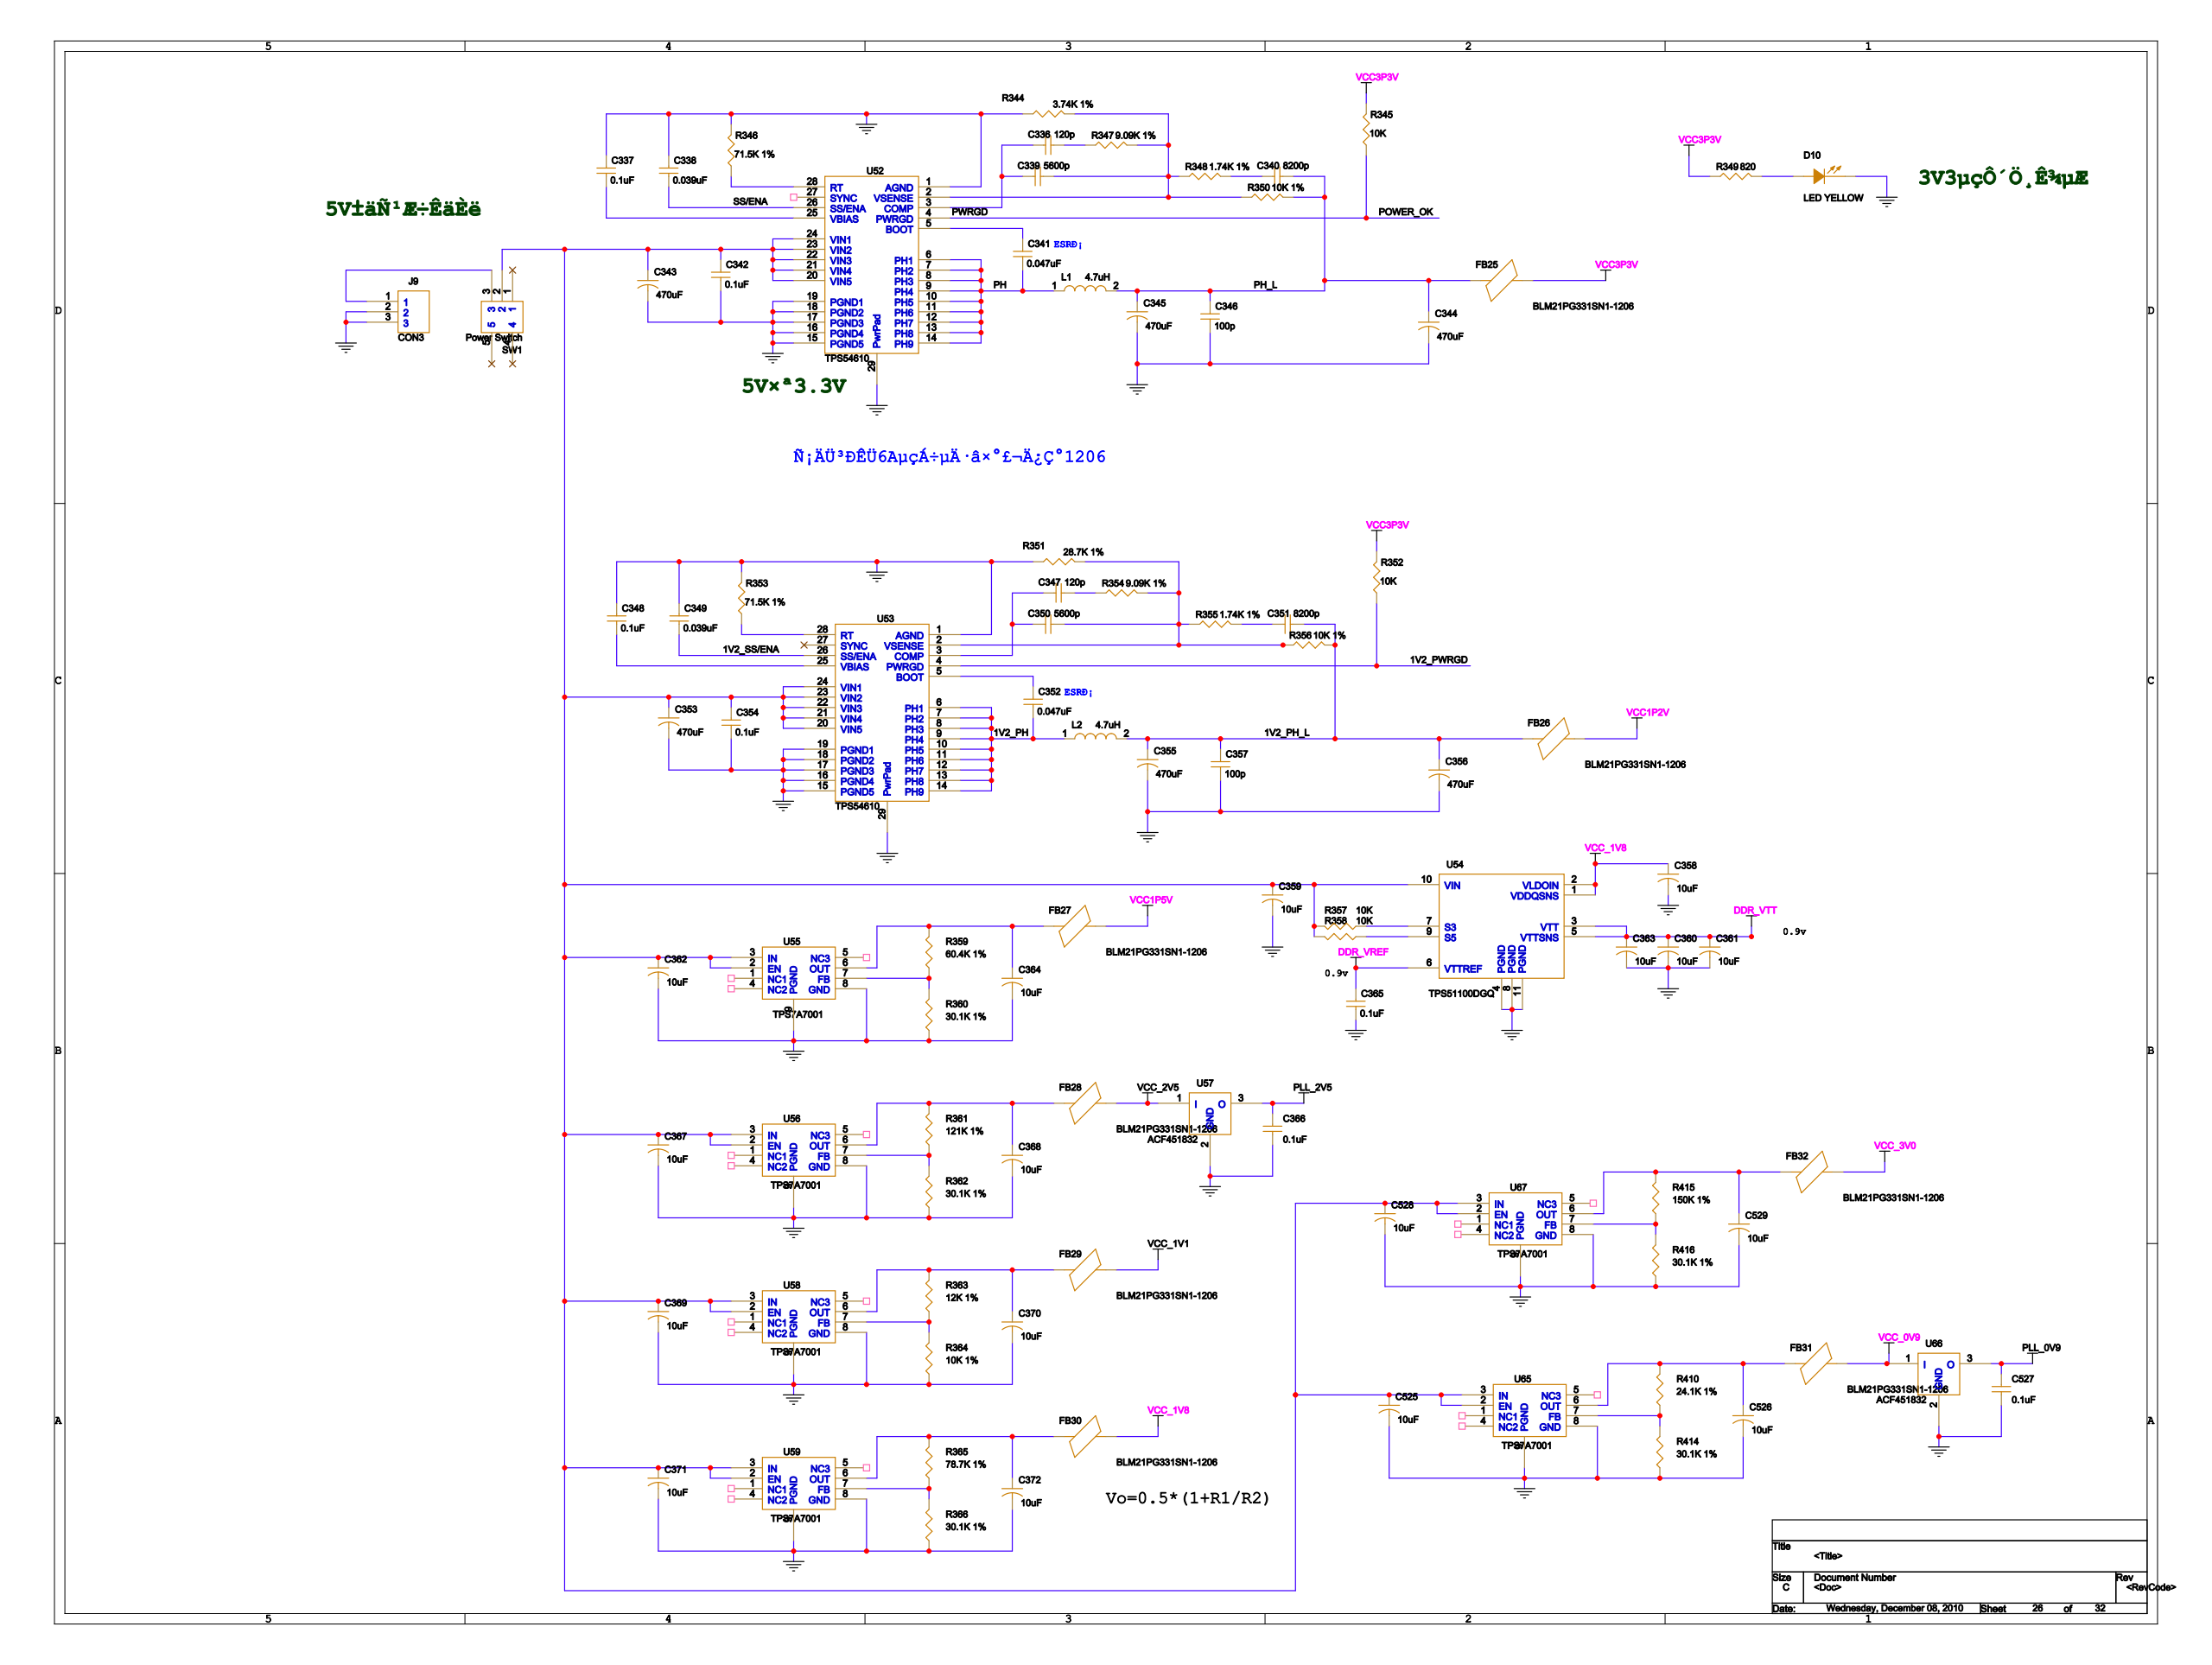Circuit board | Cadence Allegro | 1001 parts | 1318 nets | one sheet of the schematic
Parts on this sheet (reference | value | footprint):
C336 | 120p | 0603
C337 | 0.1uF | 0603
C338 | 0.039uF | 0603
C339 | 5600p | 0603
C340 | 8200p | 0603
C341 | 0.047uF | 0603
C342 | 0.1uF | 0603
C343 | 470uF | C7343
C344 | 470uF | C7343
C345 | 470uF | C7343
C346 | 100p | 0603
C347 | 120p | 0603
C348 | 0.1uF | 0603
C349 | 0.039uF | 0603
C350 | 5600p | 0603
C351 | 8200p | 0603
C352 | 0.047uF | 0603
C353 | 470uF | C7343
C354 | 0.1uF | 0603
C355 | 470uF | C7343
C356 | 470uF | C7343
C357 | 100p | 0603
C358 | 10uF | C3216
C359 | 10uF | C3216
C360 | 10uF | C3216
C361 | 10uF | C3216
C362 | 10uF | C3216
C363 | 10uF | C3216
C364 | 10uF | C3216
C365 | 0.1uF | 0603
C366 | 0.1uF | 0603
C367 | 10uF | C3216
C368 | 10uF | C3216
C369 | 10uF | C3216
C370 | 10uF | C3216
C371 | 10uF | C3216
C372 | 10uF | C3216
FB25 | BLM21PG331SN1-1206 | 1210
FB26 | BLM21PG331SN1-1206 | 1210
FB27 | BLM21PG331SN1-1206 | C1206
FB28 | BLM21PG331SN1-1206 | C1206
FB29 | BLM21PG331SN1-1206 | C1206
FB30 | BLM21PG331SN1-1206 | C1206
J9 | CON3 | CON_POWER
L1 | 4.7uH | INC5A
L2 | 4.7uH | INC5A
R344 | 3.74K 1% | 0603
R345 | 10K | 0603
R346 | 71.5K 1% | 0603
R347 | 9.09K 1% | 0603
R348 | 1.74K 1% | 0603
R349 | 820 | 0603
R350 | 10K 1% | 0603
R351 | 28.7K 1% | 0603
R352 | 10K | 0603
R353 | 71.5K 1% | 0603
R354 | 9.09K 1% | 0603
R355 | 1.74K 1% | 0603
R356 | 10K 1% | 0603
R357 | 10K | 0603
R358 | 10K | 0603
R359 | 150K 1% | 0603
R360 | 30K 1% | 0603
R361 | 121K 1% | 0603
R362 | 30.1K 1% | 0603
R363 | 12K 1% | 0603
R364 | 10K 1% | 0603
R365 | 78.7K 1% | 0603
R366 | 30.1K 1% | 0603
R410 | 2K 1% | 0603
SW1 | Power Switch | SW1
U52 | TPS54610 | TPS54610
U53 | TPS54610 | TPS54610
U54 | TPS51100DGQ | 10-MSOP-POWERPAD
U55 | TPS7A7001 | SOIC-8
U56 | TPS7A7001 | SOIC-8
U57 | ACF451832 | EMI_FILTER
U58 | TPS7A7001 | SOIC-8
U59 | TPS7A7001 | SOIC-8
Nets of these parts (net: part-pin ...):
GND: C337-1 C338-1 C342-2 C343-2 C344-2 C345-2 C346-2 C348-1 C349-1 C353-2 C354-2 C355-2 C356-2 C357-2 C358-2 C359-2 C360-2 C361-2 C362-2 C363-2 C364-2 C365-2 C366-2 C367-2 C368-2 C369-2 C370-2 C371-2 C372-2 J9-2 J9-3 R344-1 R346-2 R351-1 R353-2 R360-1 R362-1 R364-1 R366-1 R410-2 U54-4 U54-8 U54-11 U55-8 U55-9 U56-8 U56-9 U57-2 U58-8 U58-9 U59-8 U59-9 U52-1 U52-15 U52-16 U52-17 U52-18 U52-19 U52-29 U53-1 U53-15 U53-16 U53-17 U53-18 U53-19 U53-29
N17013829: R410-1
VCC_1V1: FB29-2
PLL_2V5: C366-1 U57-3
VCC3P0V: FB27-2
VCC_2V5: FB28-2 U57-1
VCC3P3V: FB25-2 R345-2 R349-1 R352-2
VCC_1V8: C358-1 FB30-2 U54-1 U54-2
DDR_VREF: C365-1 U54-6
DDR_VTT: C360-1 C361-1 C363-1 U54-3 U54-5
PH_L: C340-2 C344-1 C345-1 C346-1 FB25-1 L1-2 R350-2
1V2_PH_L: C351-2 C355-1 C356-1 C357-1 FB26-1 L2-2 R356-2
VCC1P2V: FB26-2
N16970881: C342-1 C343-1 C353-1 C354-1 C359-1 C362-1 C367-1 C369-1 C371-1 R357-2 R358-2 SW1-2 U54-10 U55-2 U55-3 U56-2 U56-3 U58-2 U58-3 U59-2 U59-3 U52-20 U52-21 U52-22 U52-23 U52-24 U53-20 U53-21 U53-22 U53-23 U53-24
N17091485: C364-1 FB27-1 R359-2 U55-6
N17092451: C368-1 FB28-1 R361-2 U56-6
N17092673: C370-1 FB29-1 R363-2 U58-6
N17464481: C372-1 FB30-1 R365-2 U59-6
N16970885: C337-2 U52-25
N16973256: C348-2 U53-25
N16970854: C336-1 C339-1 U52-3
N16970842: C336-2 R347-1
N16973241: C347-1 C350-1 U53-3
N16973243: C347-2 R354-1
SS/ENA: C338-2 U52-26
1V2_SS/ENA: C349-2 U53-26
N16970891: C339-2 R344-2 R347-2 R348-1 R350-1 U52-2
N16973268: C350-2 R351-2 R354-2 R355-1 R356-1 U53-2
N16970866: C340-1 R348-2
N16973247: C351-1 R355-2
N16970864: C341-1 U52-5
PH: C341-2 L1-1 U52-6 U52-7 U52-8 U52-9 U52-10 U52-11 U52-12 U52-13 U52-14
N16973245: C352-1 U53-5
1V2_PH: C352-2 L2-1 U53-6 U53-7 U53-8 U53-9 U53-10 U53-11 U53-12 U53-13 U53-14
N16971257: R349-2
N16971241: J9-1 SW1-3
POWER_OK: R345-1 U52-4
1V2_PWRGD: R352-1 U53-4
N17505071: R357-1 U54-7
N17505078: R358-1 U54-9
N16971356: R346-1 U52-28
N16973451: R353-1 U53-28
N17092679: R363-1 R364-2 U58-7
N17091477: R359-1 R360-2 U55-7
N17092453: R361-1 R362-2 U56-7
N17464487: R365-1 R366-2 U59-7